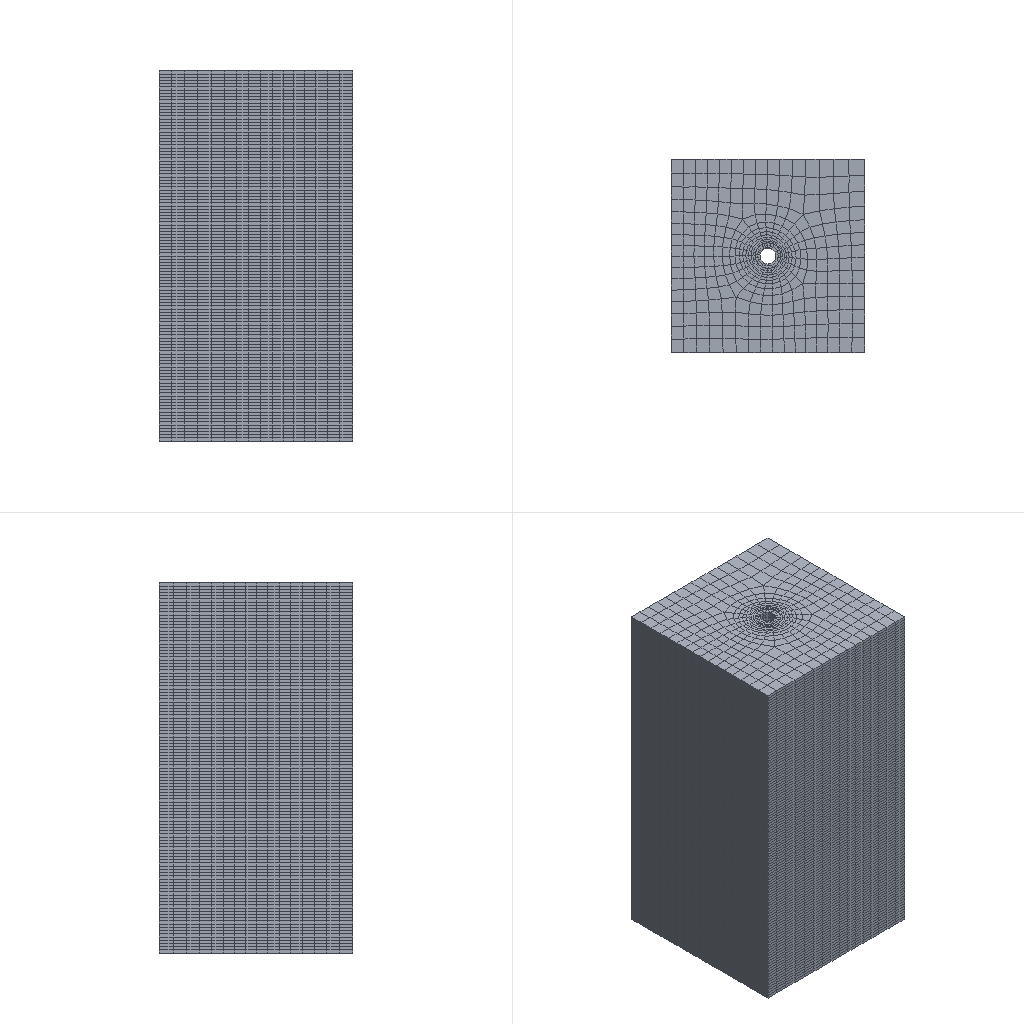Simulation study | abaqus
Set-up summary:
category,name,step,type,value,unit,region
solver,abaqus
solver,version,,,Abaqus/Explicit 2020
units,not stated in the deck,,not stated
analysis,deck,,transient,transient
load_step,Step-1,Step-1,transient,nlgeom=True
contact,interactions,,,general=0 pairs=1 ties=0
load_step,requested,,,1
mesh,nodes,,,60540
mesh,elements,,,52504
element_type,C3D8R,,solid,52504
load,load commands in deck,,count,1
bc,support commands in deck,,count,3
material,BASE,,in results
material,SUIDAO,,in results
check,setup vs results,,match,"per instance, exact: element labels, types and connectivity; labels of the nodes the elements use; coordinates of those nodes at SINGLE_PRECISION in 2 of 2 instance(s)"
Abaqus input file, long lists of numbers shortened:
*Heading
** Job name: Job-1 Model name: Model-1
** Generated by: Abaqus/CAE 2020
*Preprint, echo=NO, model=NO, history=NO, contact=NO
**
** PARTS
**
*Part, name=base
*Node
      1,          68.,         -60.,         115.
      2,         120.,        -120.,         115.
** (52882 more lines like these left out)
*Element, type=C3D8R
   1,   890,   891,   980,   968, 11904, 11905, 11994, 11982
   2,   891,   879,   892,   980, 11905, 11893, 11906, 11994
** (47442 more lines like these left out)
*Nset, nset=Set-1, generate
     1,  52884,      1
*Elset, elset=Set-1, generate
     1,  47444,      1
** Section: base
*Solid Section, elset=Set-1, material=base
,
*End Part
**
*Part, name=cq
*Node
      1,  -4.971,  0.5373,           0.
      2,    -7.968,  0.7159,           0.
** (7654 more lines like these left out)
*Element, type=C3D8R
   1,   67,   75,  115,   84,    1,    9,   49,   18
   2,   75,   68,   76,  115,    9,    2,   10,   49
** (5058 more lines like these left out)
*Nset, nset=Set-1, generate
    1,  7656,     1
*Elset, elset=Set-1, generate
    1,  5060,     1
** Section: cq
*Solid Section, elset=Set-1, material=suidao
,
*End Part
**
**
** ASSEMBLY
**
*Assembly, name=Assembly
**
*Instance, name=base-1, part=base
*End Instance
**
*Instance, name=cq-1, part=cq
         60.,         -60.,           0.
*End Instance
**
*Nset, nset=Set-1, instance=base-1
     2,     4,    17,    20,    24,    25,    92,    93,    94,    95,    96,    97,    98,    99,   100,   101
   102,   103,   104,   105,   106,   505,   506,   507,   508,   509,   510,   511,   512,   513,   514,   515
** (61 more lines like these left out)
*Elset, elset=Set-1, instance=base-1
 23949, 23950, 23951, 23952, 23953, 23954, 23955, 23956, 23957, 24053, 24056, 24059, 24060, 24068, 24076, 24084
 24358, 24359, 24360, 24361, 24362, 24363, 24364, 24365, 24366, 24462, 24465, 24468, 24469, 24477, 24485, 24493
** (56 more lines like these left out)
*Nset, nset=Set-2, instance=base-1
    17,    20,    24,    25,   607,   608,   609,   610,   611,   612,   613,   614,   615,   616,   617,   618
   619,   620,   621,   622,   623,   624,   625,   626,   627,   628,   629,   630,   631,   632,   633,   634
** (47 more lines like these left out)
*Elset, elset=Set-2, instance=base-1
 29266, 29267, 29268, 29269, 29270, 29271, 29272, 29273, 29274, 29370, 29373, 29376, 29377, 29385, 29393, 29401
 29675, 29676, 29677, 29678, 29679, 29680, 29681, 29682, 29683, 29779, 29782, 29785, 29786, 29794, 29802, 29810
** (43 more lines like these left out)
*Nset, nset=Set-3, instance=base-1
     2,     3,     4,     5,     7,     8,     9,    10,    12,    13,    14,    15,    17,    18,    19,    20
    22,    23,    24,    25,    50,    51,    52,    53,    54,    55,    56,    57,    58,    59,    60,    61
** (232 more lines like these left out)
*Elset, elset=Set-3, instance=base-1
    67,    70,    73,    76,   209,   218,   227,   250,   251,   252,   253,   254,   255,   256,   362,   363
   364,   365,   366,   367,   368,   369,   381,   385,   389,   393,   397,   401,   405,   409,   476,   479
** (216 more lines like these left out)
*Nset, nset=Set-4, instance=base-1
   11,   12,   13,   14,   15,   21,   22,   23,   24,   25,  412,  413,  414,  415,  416,  417
  418,  419,  420,  421,  422,  423,  424,  425,  426,  427,  428,  429,  430,  431,  432,  433
** (55 more lines like these left out)
*Nset, nset=Set-4, instance=cq-1
    1,    2,    3,    4,    5,    6,    7,    8,    9,   10,   11,   12,   13,   14,   15,   16
   17,   18,   19,   20,   21,   22,   23,   24,   25,   26,   27,   28,   29,   30,   31,   32
** (7 more lines like these left out)
*Elset, elset=Set-4, instance=base-1
 23314, 23315, 23316, 23317, 23318, 23319, 23320, 23321, 23322, 23323, 23324, 23325, 23326, 23327, 23328, 23329
 23330, 23331, 23332, 23333, 23334, 23335, 23336, 23337, 23338, 23339, 23340, 23341, 23342, 23343, 23344, 23345
** (50 more lines like these left out)
*Elset, elset=Set-4, instance=cq-1
    1,    2,    3,    4,    5,    6,    7,    8,    9,   10,   11,   12,   13,   14,   15,   16
   17,   18,   19,   20,   21,   22,   23,   24,   25,   26,   27,   28,   29,   30,   31,   32
** (4 more lines like these left out)
*Elset, elset=_Surf-3_S6, internal, instance=base-1
  5553,  5560,  5567,  5687,  5689,  5691,  5693,  5962,  5969,  5976,  6096,  6098,  6100,  6102,  6371,  6378
  6385,  6505,  6507,  6509,  6511,  6780,  6787,  6794,  6914,  6916,  6918,  6920,  7189,  7196,  7203,  7323
** (18 more lines like these left out)
*Elset, elset=_Surf-3_S4, internal, instance=base-1
  5575,  5577,  5579,  5581,  5984,  5986,  5988,  5990,  6393,  6395,  6397,  6399,  6802,  6804,  6806,  6808
  7211,  7213,  7215,  7217,  7620,  7622,  7624,  7626,  8029,  8031,  8033,  8035,  8438,  8440,  8442,  8444
** (10 more lines like these left out)
*Elset, elset=_Surf-3_S3, internal, instance=base-1
  5695,  5696,  5697,  5698,  6104,  6105,  6106,  6107,  6513,  6514,  6515,  6516,  6922,  6923,  6924,  6925
  7331,  7332,  7333,  7334,  7740,  7741,  7742,  7743,  8149,  8150,  8151,  8152,  8558,  8559,  8560,  8561
** (10 more lines like these left out)
*Surface, type=ELEMENT, name=Surf-3
_Surf-3_S6, S6
_Surf-3_S4, S4
_Surf-3_S3, S3
*Elset, elset=_Surf-4_S6, internal, instance=base-1
   236,   243,   250,   370,   372,   374,   376,   645,   652,   659,   779,   781,   783,   785,  1054,  1061
  1068,  1188,  1190,  1192,  1194,  1463,  1470,  1477,  1597,  1599,  1601,  1603,  1872,  1879,  1886,  2006
** (24 more lines like these left out)
*Elset, elset=_Surf-4_S4, internal, instance=base-1
   258,   260,   262,   264,   667,   669,   671,   673,  1076,  1078,  1080,  1082,  1485,  1487,  1489,  1491
  1894,  1896,  1898,  1900,  2303,  2305,  2307,  2309,  2712,  2714,  2716,  2718,  3121,  3123,  3125,  3127
** (13 more lines like these left out)
*Elset, elset=_Surf-4_S3, internal, instance=base-1
   378,   379,   380,   381,   787,   788,   789,   790,  1196,  1197,  1198,  1199,  1605,  1606,  1607,  1608
  2014,  2015,  2016,  2017,  2423,  2424,  2425,  2426,  2832,  2833,  2834,  2835,  3241,  3242,  3243,  3244
** (13 more lines like these left out)
*Surface, type=ELEMENT, name=Surf-4
_Surf-4_S6, S6
_Surf-4_S4, S4
_Surf-4_S3, S3
*Elset, elset=_m_Surf-1_S4, internal, instance=base-1
    16,    24,    89,    98,   107,   159,   168,   284,   292,   300,   308,   425,   433,   498,   507,   516
   568,   577,   693,   701,   709,   717,   834,   842,   907,   916,   925,   977,   986,  1102,  1110,  1118
** (38 more lines like these left out)
*Elset, elset=_m_Surf-1_S3, internal, instance=base-1
    25,    26,    27,    28,   108,   109,   110,   111,   169,   170,   171,   172,   309,   310,   434,   435
   436,   437,   517,   518,   519,   520,   578,   579,   580,   581,   718,   719,   843,   844,   845,   846
** (49 more lines like these left out)
*Elset, elset=_m_Surf-1_S5, internal, instance=base-1
 23738, 23746, 23811, 23820, 23829, 23881, 23890, 24006, 24014, 24022, 24030, 24147, 24155, 24220, 24229, 24238
 24290, 24299, 24415, 24423, 24431, 24439, 24556, 24564, 24629, 24638, 24647, 24699, 24708, 24824, 24832, 24840
** (38 more lines like these left out)
*Elset, elset=_m_Surf-1_S6, internal, instance=base-1
 23747, 23748, 23749, 23750, 23830, 23831, 23832, 23833, 23891, 23892, 23893, 23894, 24031, 24032, 24156, 24157
 24158, 24159, 24239, 24240, 24241, 24242, 24300, 24301, 24302, 24303, 24440, 24441, 24565, 24566, 24567, 24568
** (49 more lines like these left out)
*Surface, type=ELEMENT, name=m_Surf-1
_m_Surf-1_S4, S4
_m_Surf-1_S3, S3
_m_Surf-1_S6, S6
_m_Surf-1_S5, S5
*Elset, elset=_s_Surf-1_S4, internal, instance=cq-1
    2,    4,    6,    8,   10,   34,   36,   38,   40,   42,   44,   46,   48,   50,   52,   54
   78,   80,   82,   84,   86,   88,   90,   92,   94,   96,   98,  122,  124,  126,  128,  130
** (78 more lines like these left out)
*Elset, elset=_s_Surf-1_S6, internal, instance=cq-1
   11,   13,   15,   17,   19,   21,   23,   25,   27,   29,   31,   55,   57,   59,   61,   63
   65,   67,   69,   71,   73,   75,   99,  101,  103,  105,  107,  109,  111,  113,  115,  117
** (78 more lines like these left out)
*Surface, type=ELEMENT, name=s_Surf-1
_s_Surf-1_S4, S4
_s_Surf-1_S6, S6
*End Assembly
*Amplitude, name=Amp-1
             0.,              0.,              1.,              1.
**
** MATERIALS
**
*Material, name=base
*Density
2600.,
*Elastic
 6e+09, 0.35
*Mohr Coulomb
45.,0.
*Mohr Coulomb Hardening
590000.,0.
*Material, name=suidao
*Density
2500.,
*Elastic
 3.1e+10, 0.25
*Mohr Coulomb
54.,0.
*Mohr Coulomb Hardening
 4.13e+06,0.
**
** INTERACTION PROPERTIES
**
*Surface Interaction, name=IntProp-1
*Friction
 0.15,
*Surface Behavior, pressure-overclosure=HARD
** ----------------------------------------------------------------
**
** STEP: Step-1
**
*Step, name=Step-1, nlgeom=YES
*Dynamic, Explicit
, 1.
*Bulk Viscosity
0.06, 1.2
**
** BOUNDARY CONDITIONS
**
** Name: BC-1 Type: 对称/反对称/完全固定
*Boundary
Set-2, ENCASTRE
** Name: BC-2 Type: 位移/转角
*Boundary
Set-3, 1, 1
** Name: BC-3 Type: 位移/转角
*Boundary
Set-4, 3, 3
**
** LOADS
**
** Name: Load-1   Type: Pressure
*Dsload, amplitude=Amp-1
Surf-4, P, 1e+07
**
** INTERACTIONS
**
** Interaction: Int-1
*Contact Pair, interaction=IntProp-1, mechanical constraint=KINEMATIC, cpset=Int-1
m_Surf-1, s_Surf-1
**
** OUTPUT REQUESTS
**
*Restart, write, number interval=1, time marks=NO
**
** FIELD OUTPUT: F-Output-1
**
*Output, field
*Node Output
CF, RF, RM, RT, U, V
*Element Output, directions=YES
CTSHR, E, LE, MISES, MISESMAX, MISESONLY, PE, PEEQ, PEEQMAX, PEEQT, PEMAG, PEQC, PRESSONLY, S, SEQUT, TSHR
YIELDPOT
*Contact Output
CDISP, CFORCE, CSTRESS, PPRESS
**
** HISTORY OUTPUT: H-Output-1
**
*Output, history, variable=PRESELECT, frequency=1
*End Step
Results summary:
result,step,Step-1,completed,increments=3017 time=1.0/1.0
result,analysis,,,transient
result,last_loadstep,,,1
result,analysis steps,,count,1
result,primary field,,,U
result,reaction total,,FX,158591116.453,model units
result,reaction total,,FY,14204004914.625,model units
result,reaction total,,FZ,-5894041871.691,model units